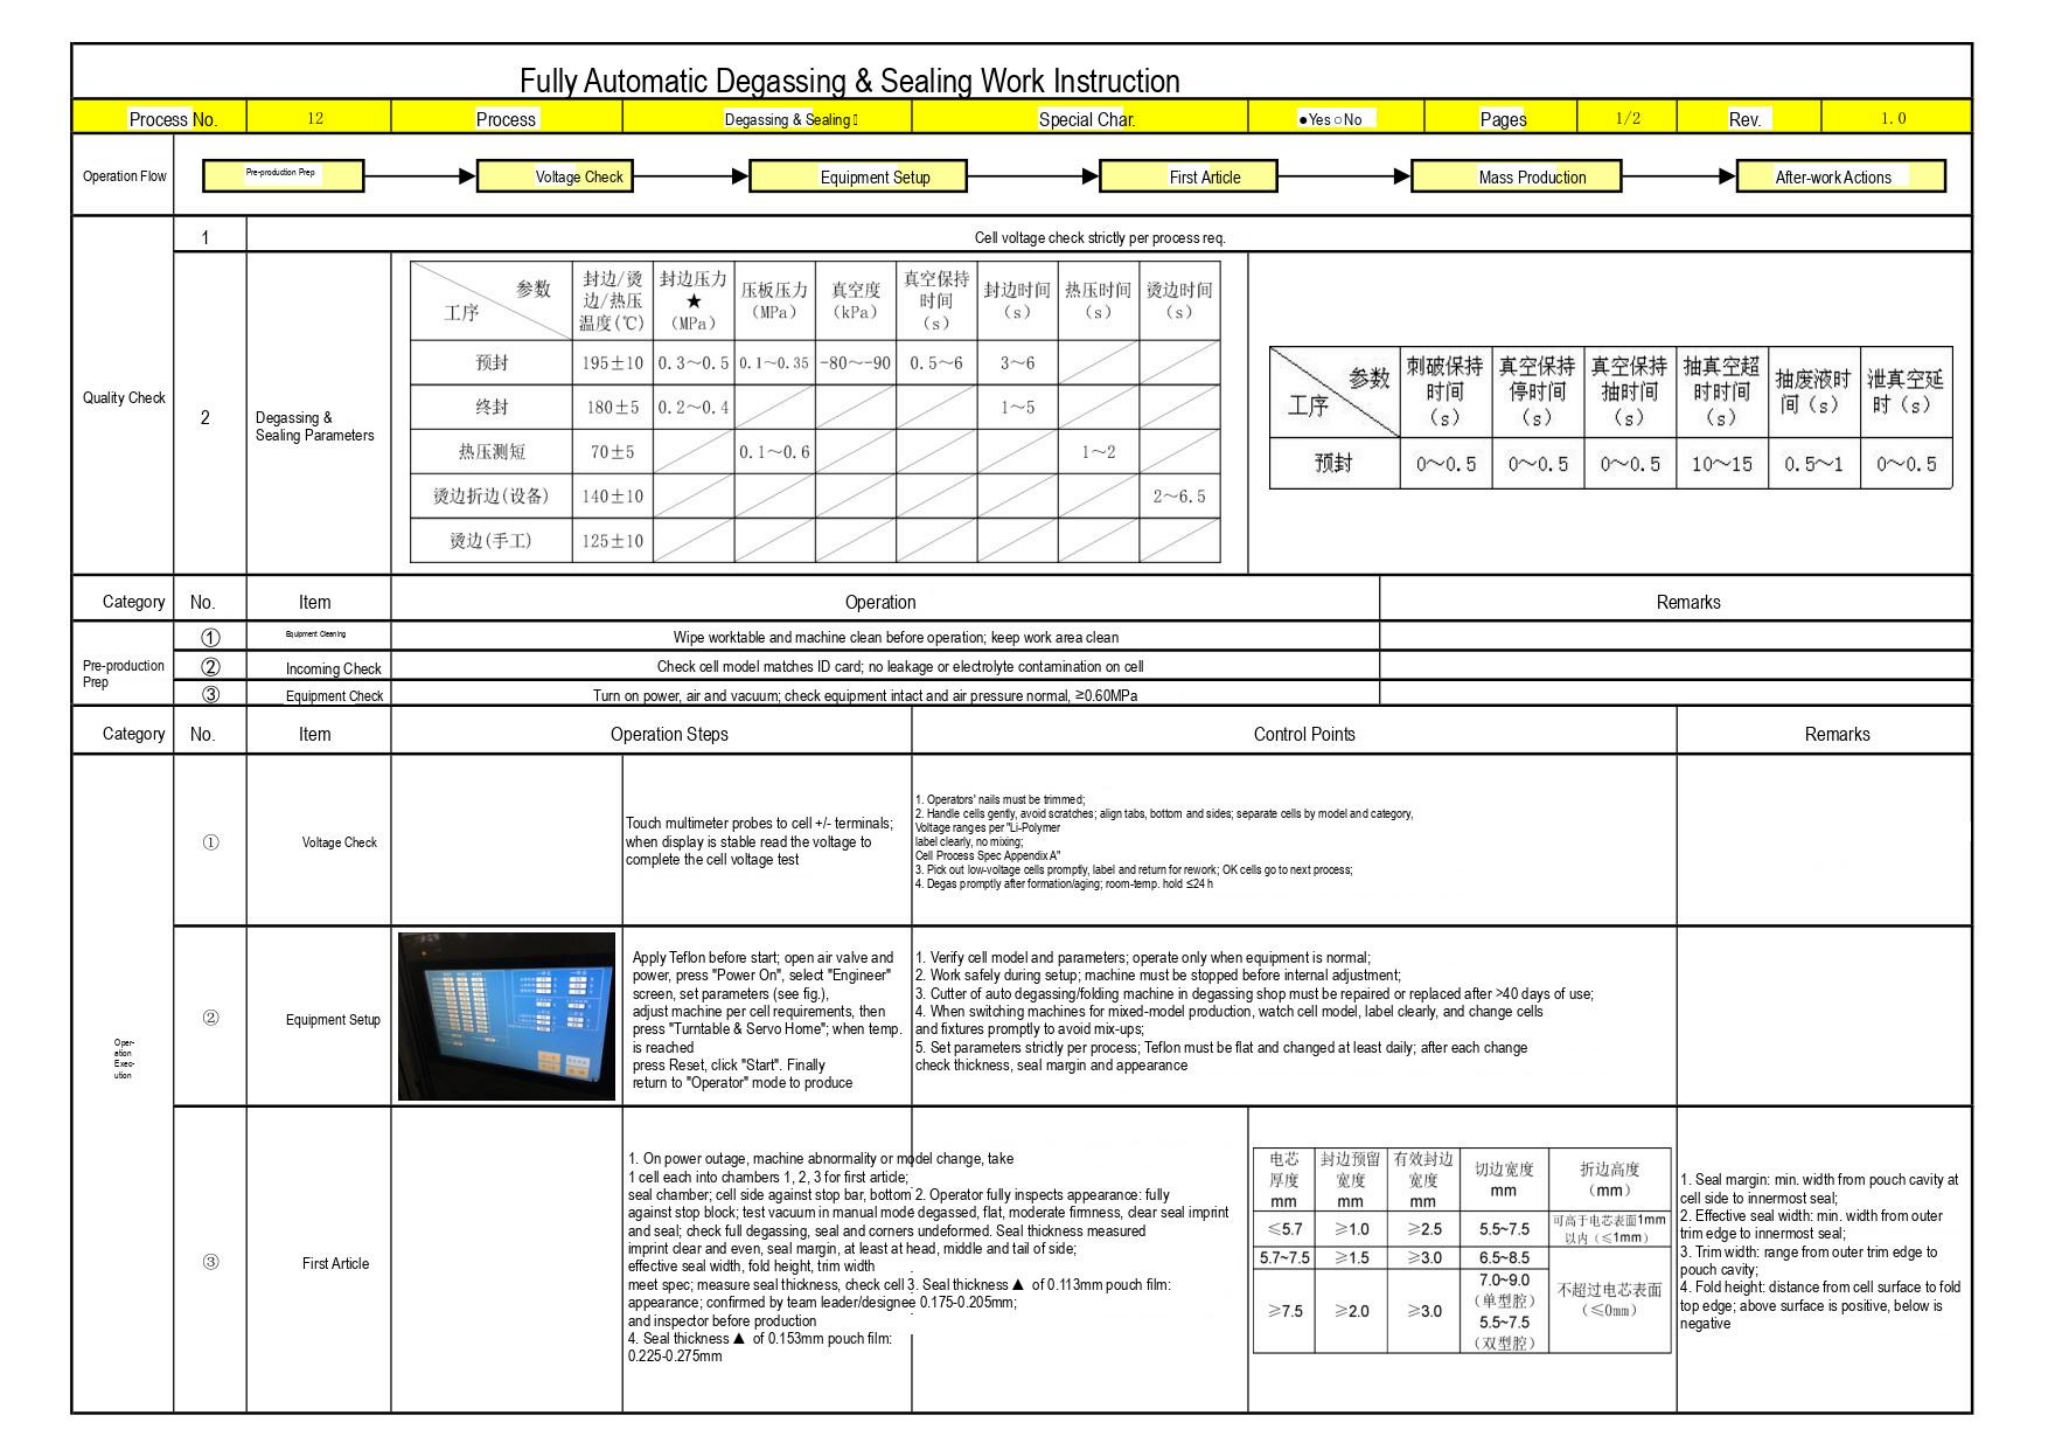# Fully Automatic Degassing & Sealing Work Instruction

| Process No. | 12 | Process | Degassing & Sealing | Special Char. | ●Yes ○No | Pages | 1/2 | Rev. | 1.0 |
|---|---|---|---|---|---|---|---|---|---|

**Operation Flow:** Pre-production Prep → Voltage Check → Equipment Setup → First Article → Mass Production → After-work Actions

**Quality Check**

| No. | Item | Content |
|---|---|---|
| 1 | | Cell voltage check strictly per process req. |
| 2 | Degassing & Sealing Parameters | (see tables below) |

| 参数 / 工序 | 封边/烫边/热压温度(℃) | 封边压力★(MPa) | 压板压力(MPa) | 真空度(kPa) | 真空保持时间(s) | 封边时间(s) | 热压时间(s) | 烫边时间(s) |
|---|---|---|---|---|---|---|---|---|
| 预封 | 195±10 | 0.3~0.5 | 0.1~0.35 | -80~-90 | 0.5~6 | 3~6 | | |
| 终封 | 180±5 | 0.2~0.4 | | | | 1~5 | | |
| 热压测短 | 70±5 | | 0.1~0.6 | | | | 1~2 | |
| 烫边折边(设备) | 140±10 | | | | | | | 2~6.5 |
| 烫边(手工) | 125±10 | | | | | | | |

| 参数 / 工序 | 刺破保持时间(s) | 真空保持停时间(s) | 真空保持抽时间(s) | 抽真空超时时间(s) | 抽废液时间(s) | 泄真空延时(s) |
|---|---|---|---|---|---|---|
| 预封 | 0~0.5 | 0~0.5 | 0~0.5 | 10~15 | 0.5~1 | 0~0.5 |

| Category | No. | Item | Operation | Remarks |
|---|---|---|---|---|
| Pre-production Prep | ① | Equipment Cleaning | Wipe worktable and machine clean before operation; keep work area clean | |
| | ② | Incoming Check | Check cell model matches ID card; no leakage or electrolyte contamination on cell | |
| | ③ | Equipment Check | Turn on power, air and vacuum; check equipment intact and air pressure normal, ≥0.60MPa | |

| Category | No. | Item | Operation Steps | Control Points | Remarks |
|---|---|---|---|---|---|
| Operation Execution | ① | Voltage Check | Touch multimeter probes to cell +/- terminals; when display is stable read the voltage to complete the cell voltage test | 1. Operators' nails must be trimmed;<br>2. Handle cells gently, avoid scratches; align tabs, bottom and sides; separate cells by model and category, Voltage ranges per "Li-Polymer label clearly, no mixing; Cell Process Spec Appendix A"<br>3. Pick out low-voltage cells promptly, label and return for rework; OK cells go to next process;<br>4. Degas promptly after formation/aging; room-temp. hold ≤24 h | |
| | ② | Equipment Setup | Apply Teflon before start; open air valve and power, press "Power On", select "Engineer" screen, set parameters (see fig.), adjust machine per cell requirements, then press "Turntable & Servo Home"; when temp. is reached press Reset, click "Start". Finally return to "Operator" mode to produce | 1. Verify cell model and parameters; operate only when equipment is normal;<br>2. Work safely during setup; machine must be stopped before internal adjustment;<br>3. Cutter of auto degassing/folding machine in degassing shop must be repaired or replaced after >40 days of use;<br>4. When switching machines for mixed-model production, watch cell model, label clearly, and change cells and fixtures promptly to avoid mix-ups;<br>5. Set parameters strictly per process; Teflon must be flat and changed at least daily; after each change check thickness, seal margin and appearance | |
| | ③ | First Article | 1. On power outage, machine abnormality or model change, take 1 cell each into chambers 1, 2, 3 for first article; seal chamber; cell side against stop bar, bottom against stop block; test vacuum in manual mode and seal; check full degassing, seal and corners imprint clear and even, seal margin, effective seal width, fold height, trim width meet spec; measure seal thickness, check cell appearance; confirmed by team leader/designee and inspector before production | 2. Operator fully inspects appearance: fully degassed, flat, moderate firmness, clear seal imprint undeformed. Seal thickness measured at least at head, middle and tail of side;<br>3. Seal thickness ▲ of 0.113mm pouch film: 0.175-0.205mm;<br>4. Seal thickness ▲ of 0.153mm pouch film: 0.225-0.275mm | 1. Seal margin: min. width from pouch cavity at cell side to innermost seal;<br>2. Effective seal width: min. width from outer trim edge to innermost seal;<br>3. Trim width: range from outer trim edge to pouch cavity;<br>4. Fold height: distance from cell surface to fold top edge; above surface is positive, below is negative |

| 电芯厚度 mm | 封边预留宽度 mm | 有效封边宽度 mm | 切边宽度 mm | 折边高度(mm) |
|---|---|---|---|---|
| ≤5.7 | ≥1.0 | ≥2.5 | 5.5~7.5 | 可高于电芯表面1mm以内(≤1mm) |
| 5.7~7.5 | ≥1.5 | ≥3.0 | 6.5~8.5 | |
| ≥7.5 | ≥2.0 | ≥3.0 | 7.0~9.0(单型腔)<br>5.5~7.5(双型腔) | 不超过电芯表面(≤0mm) |
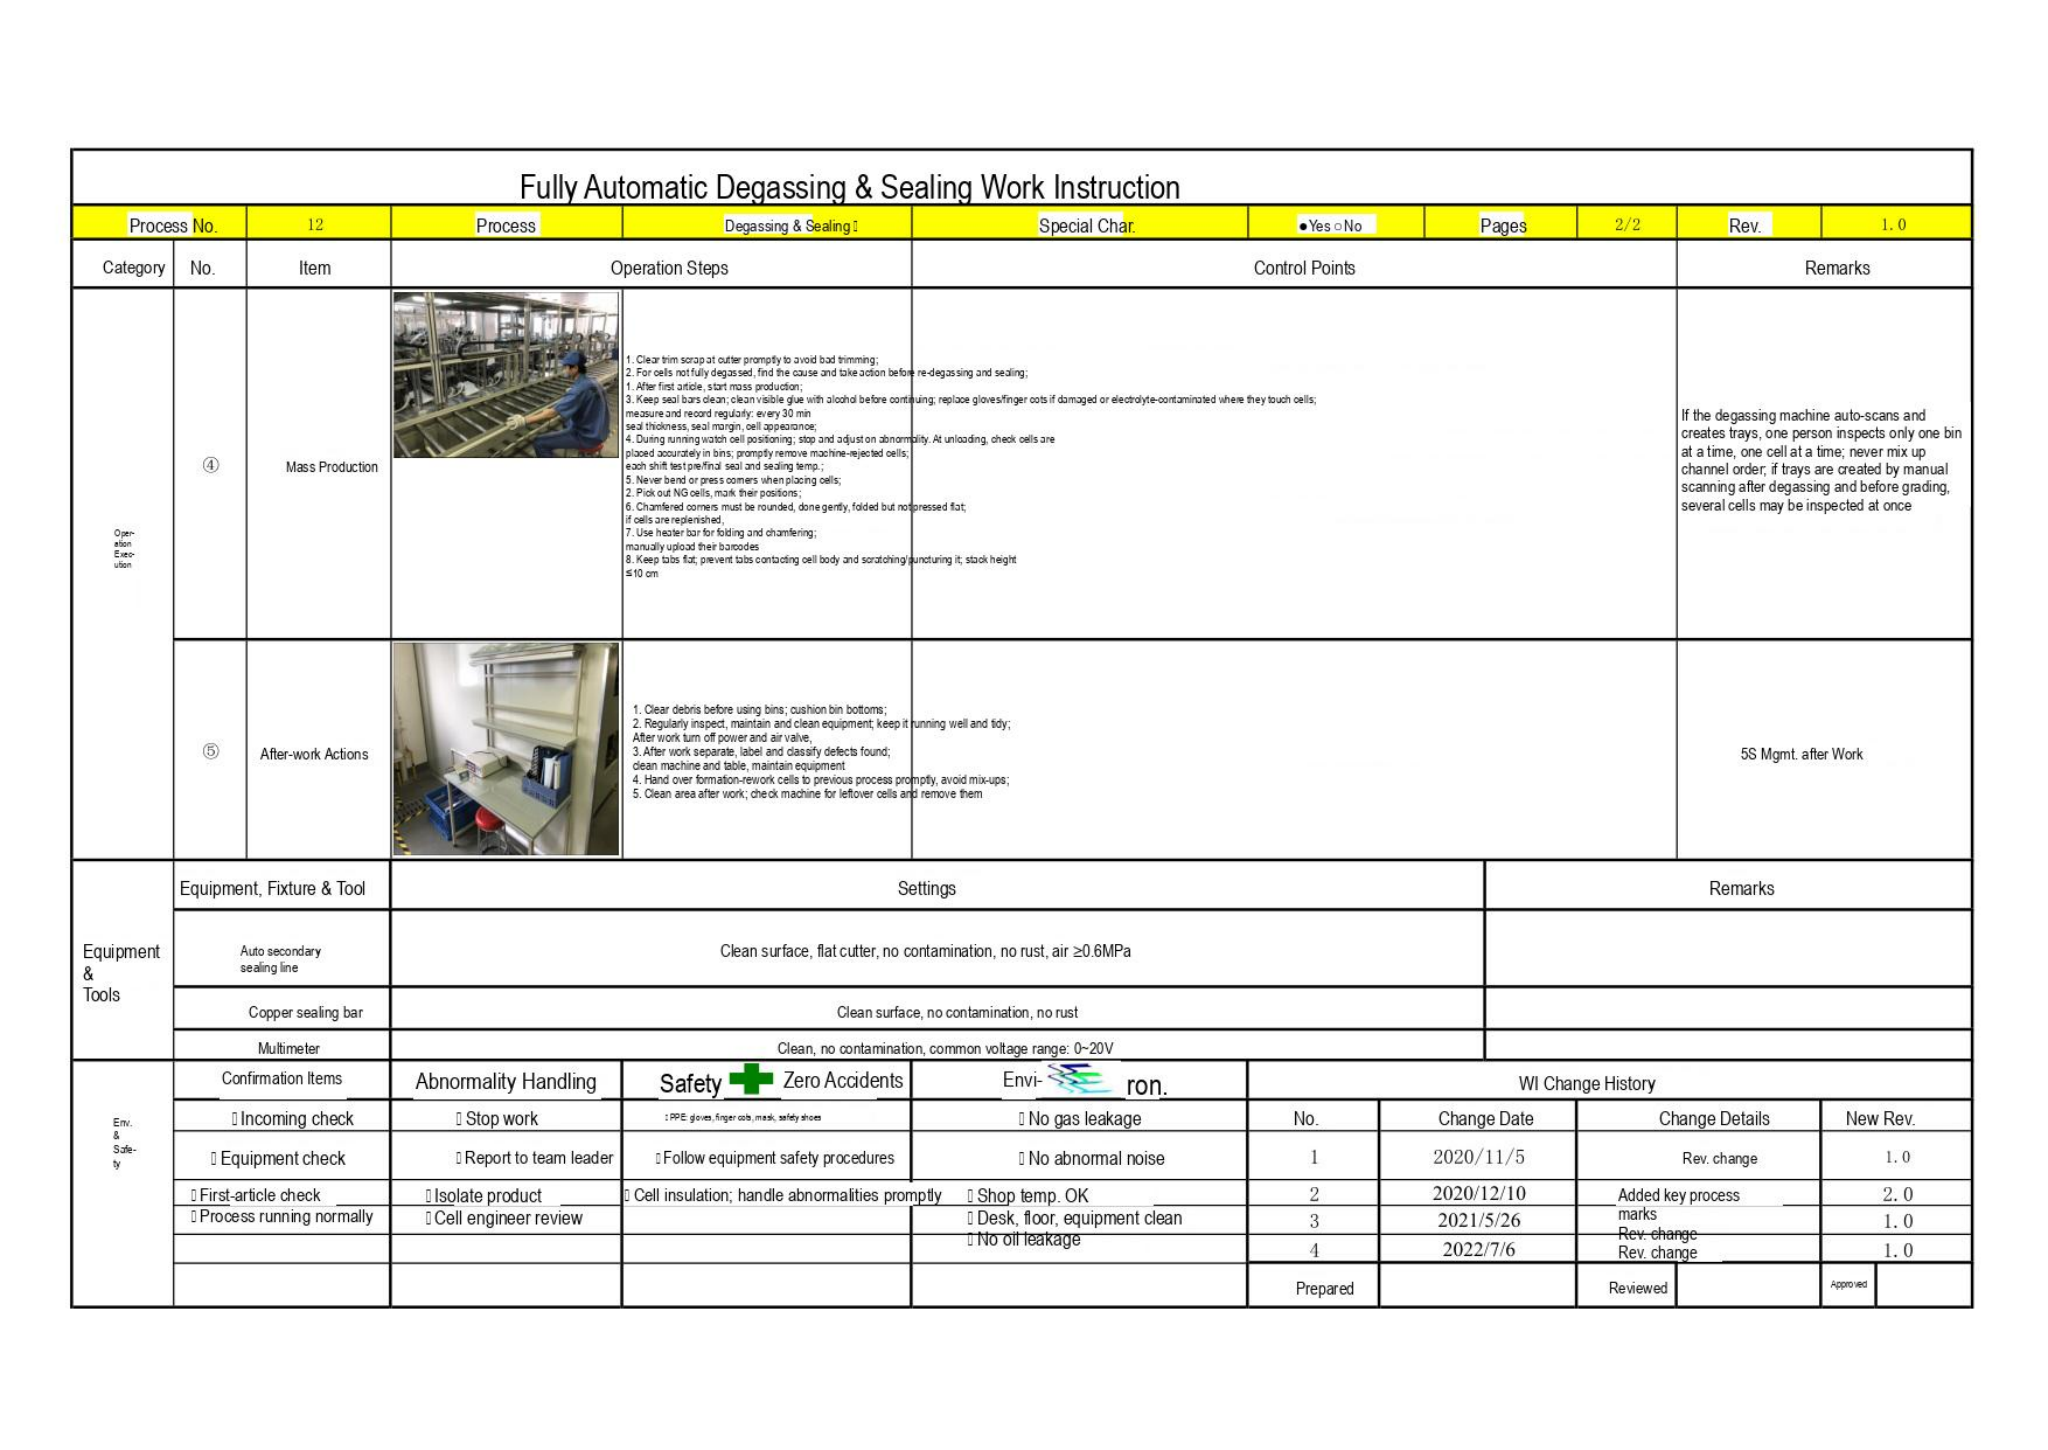# Fully Automatic Degassing & Sealing Work Instruction

| Process No. | 12 | Process | Degassing & Sealing | Special Char. | ●Yes ○No | Pages | 2/2 | Rev. | 1.0 |
|---|---|---|---|---|---|---|---|---|---|

| Category | No. | Item | Operation Steps | Control Points | Remarks |
|---|---|---|---|---|---|
| Oper-ation Exec-ution | ④ | Mass Production | 1. Clear trim scrap at cutter promptly to avoid bad trimming;<br>2. For cells not fully degassed, find the cause and take action before re-degassing and sealing;<br>1. After first article, start mass production;<br>3. Keep seal bars clean; clean visible glue with alcohol before continuing; replace gloves/finger cots if damaged or electrolyte-contaminated where they touch cells;<br>measure and record regularly: every 30 min<br>seal thickness, seal margin, cell appearance;<br>4. During running watch cell positioning; stop and adjust on abnormality. At unloading, check cells are<br>placed accurately in bins; promptly remove machine-rejected cells;<br>each shift test pre/final seal and sealing temp.;<br>5. Never bend or press corners when placing cells;<br>2. Pick out NG cells, mark their positions;<br>6. Chamfered corners must be rounded, done gently, folded but not pressed flat;<br>if cells are replenished,<br>7. Use heater bar for folding and chamfering;<br>manually upload their barcodes<br>8. Keep tabs flat; prevent tabs contacting cell body and scratching/puncturing it; stack height<br>≤10 cm | | If the degassing machine auto-scans and creates trays, one person inspects only one bin at a time, one cell at a time; never mix up channel order; if trays are created by manual scanning after degassing and before grading, several cells may be inspected at once |
| | ⑤ | After-work Actions | 1. Clear debris before using bins; cushion bin bottoms;<br>2. Regularly inspect, maintain and clean equipment; keep it running well and tidy;<br>After work turn off power and air valve,<br>3. After work separate, label and classify defects found;<br>clean machine and table, maintain equipment<br>4. Hand over formation-rework cells to previous process promptly, avoid mix-ups;<br>5. Clean area after work; check machine for leftover cells and remove them | | 5S Mgmt. after Work |

| Category | Equipment, Fixture & Tool | Settings | Remarks |
|---|---|---|---|
| Equipment & Tools | Auto secondary sealing line | Clean surface, flat cutter, no contamination, no rust, air ≥0.6MPa | |
| | Copper sealing bar | Clean surface, no contamination, no rust | |
| | Multimeter | Clean, no contamination, common voltage range: 0~20V | |

| Category | Confirmation Items | Abnormality Handling | Safety Zero Accidents | Envi- ron. | WI Change History | | | |
|---|---|---|---|---|---|---|---|---|
| Env. & Safe-ty | Incoming check | Stop work | PPE: gloves, finger cots, mask, safety shoes | No gas leakage | No. | Change Date | Change Details | New Rev. |
| | Equipment check | Report to team leader | Follow equipment safety procedures | No abnormal noise | 1 | 2020/11/5 | Rev. change | 1.0 |
| | First-article check | Isolate product | Cell insulation; handle abnormalities promptly | Shop temp. OK | 2 | 2020/12/10 | Added key process marks | 2.0 |
| | Process running normally | Cell engineer review | | Desk, floor, equipment clean | 3 | 2021/5/26 | Rev. change | 1.0 |
| | | | | No oil leakage | 4 | 2022/7/6 | Rev. change | 1.0 |
| | | | | | Prepared | | Reviewed | Approved |